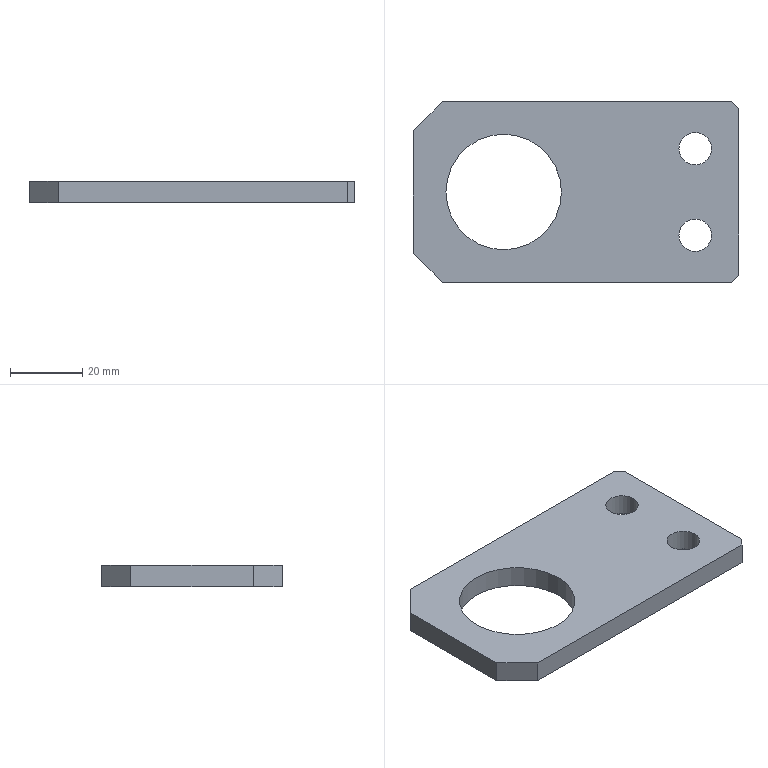Part | NX | features solid 2 | 1 solid | 13 faces | box 90.05 x 50 x 6 mm | volume 21018 mm3 | plane 10 | cylinder 3 | commonest cylinder face diameters 9 x2 32 x1
STEP:
#1=CARTESIAN_POINT('',(1617.788,161.279,-54.));
#2=VERTEX_POINT('',#1);
#3=CARTESIAN_POINT('',(1697.838,161.279,-54.));
#4=VERTEX_POINT('',#3);
#5=CARTESIAN_POINT('',(1655.838,161.279,-54.));
#6=DIRECTION('',(1.,0.,0.));
#7=VECTOR('',#6,1000.);
#8=LINE('',#5,#7);
#9=EDGE_CURVE('',#2,#4,#8,.T.);
#10=ORIENTED_EDGE('',*,*,#9,.F.);
#11=CARTESIAN_POINT('',(1609.788,153.279,-54.));
#12=VERTEX_POINT('',#11);
#13=CARTESIAN_POINT('',(1623.788,167.279,-54.));
#14=DIRECTION('',(0.7071,0.7071,0.));
#15=VECTOR('',#14,1000.);
#16=LINE('',#13,#15);
#17=EDGE_CURVE('',#2,#12,#16,.F.);
#18=ORIENTED_EDGE('',*,*,#17,.T.);
#19=CARTESIAN_POINT('',(1609.788,119.279,-54.));
#20=VERTEX_POINT('',#19);
#21=CARTESIAN_POINT('',(1609.788,136.279,-54.));
#22=DIRECTION('',(0.,1.,0.));
#23=VECTOR('',#22,1000.);
#24=LINE('',#21,#23);
#25=EDGE_CURVE('',#20,#12,#24,.T.);
#26=ORIENTED_EDGE('',*,*,#25,.F.);
#27=CARTESIAN_POINT('',(1617.788,111.279,-54.));
#28=VERTEX_POINT('',#27);
#29=CARTESIAN_POINT('',(1623.788,105.279,-54.));
#30=DIRECTION('',(-0.7071,0.7071,0.));
#31=VECTOR('',#30,1000.);
#32=LINE('',#29,#31);
#33=EDGE_CURVE('',#20,#28,#32,.F.);
#34=ORIENTED_EDGE('',*,*,#33,.T.);
#35=CARTESIAN_POINT('',(1697.838,111.279,-54.));
#36=VERTEX_POINT('',#35);
#37=CARTESIAN_POINT('',(1655.838,111.279,-54.));
#38=DIRECTION('',(-1.,0.,0.));
#39=VECTOR('',#38,1000.);
#40=LINE('',#37,#39);
#41=EDGE_CURVE('',#36,#28,#40,.T.);
#42=ORIENTED_EDGE('',*,*,#41,.F.);
#43=CARTESIAN_POINT('',(1699.838,113.279,-54.));
#44=VERTEX_POINT('',#43);
#45=CARTESIAN_POINT('',(1688.838,102.279,-54.));
#46=DIRECTION('',(-0.7071,-0.7071,0.));
#47=VECTOR('',#46,1000.);
#48=LINE('',#45,#47);
#49=EDGE_CURVE('',#36,#44,#48,.F.);
#50=ORIENTED_EDGE('',*,*,#49,.T.);
#51=CARTESIAN_POINT('',(1699.838,159.279,-54.));
#52=VERTEX_POINT('',#51);
#53=CARTESIAN_POINT('',(1699.838,136.279,-54.));
#54=DIRECTION('',(0.,-1.,0.));
#55=VECTOR('',#54,1000.);
#56=LINE('',#53,#55);
#57=EDGE_CURVE('',#52,#44,#56,.T.);
#58=ORIENTED_EDGE('',*,*,#57,.F.);
#59=CARTESIAN_POINT('',(1688.838,170.279,-54.));
#60=DIRECTION('',(0.7071,-0.7071,0.));
#61=VECTOR('',#60,1000.);
#62=LINE('',#59,#61);
#63=EDGE_CURVE('',#52,#4,#62,.F.);
#64=ORIENTED_EDGE('',*,*,#63,.T.);
#65=EDGE_LOOP('',(#10,#18,#26,#34,#42,#50,#58,#64));
#66=FACE_BOUND('',#65,.T.);
#67=CARTESIAN_POINT('',(1683.338,124.279,-54.));
#68=VERTEX_POINT('',#67);
#69=CARTESIAN_POINT('',(1687.838,124.279,-54.));
#70=DIRECTION('',(0.,0.,-1.));
#71=DIRECTION('',(-1.,0.,0.));
#72=AXIS2_PLACEMENT_3D('',#69,#70,#71);
#73=CIRCLE('',#72,4.5);
#74=EDGE_CURVE('',#68,#68,#73,.T.);
#75=ORIENTED_EDGE('',*,*,#74,.T.);
#76=EDGE_LOOP('',(#75));
#77=FACE_BOUND('',#76,.T.);
#78=CARTESIAN_POINT('',(1683.338,148.279,-54.));
#79=VERTEX_POINT('',#78);
#80=CARTESIAN_POINT('',(1687.838,148.279,-54.));
#81=DIRECTION('',(0.,0.,-1.));
#82=DIRECTION('',(-1.,0.,0.));
#83=AXIS2_PLACEMENT_3D('',#80,#81,#82);
#84=CIRCLE('',#83,4.5);
#85=EDGE_CURVE('',#79,#79,#84,.T.);
#86=ORIENTED_EDGE('',*,*,#85,.T.);
#87=EDGE_LOOP('',(#86));
#88=FACE_BOUND('',#87,.T.);
#89=CARTESIAN_POINT('',(1618.788,136.279,-54.));
#90=VERTEX_POINT('',#89);
#91=CARTESIAN_POINT('',(1634.788,136.279,-54.));
#92=DIRECTION('',(0.,0.,-1.));
#93=DIRECTION('',(-1.,0.,0.));
#94=AXIS2_PLACEMENT_3D('',#91,#92,#93);
#95=CIRCLE('',#94,16.);
#96=EDGE_CURVE('',#90,#90,#95,.T.);
#97=ORIENTED_EDGE('',*,*,#96,.T.);
#98=EDGE_LOOP('',(#97));
#99=FACE_BOUND('',#98,.T.);
#100=CARTESIAN_POINT('',(1655.838,136.279,-54.));
#101=DIRECTION('',(0.,0.,1.));
#102=DIRECTION('',(1.,0.,0.));
#103=AXIS2_PLACEMENT_3D('',#100,#101,#102);
#104=PLANE('',#103);
#105=ADVANCED_FACE('',(#66,#77,#88,#99),#104,.T.);
#106=ORIENTED_EDGE('',*,*,#41,.T.);
#107=CARTESIAN_POINT('',(1617.788,111.279,-60.));
#108=VERTEX_POINT('',#107);
#109=CARTESIAN_POINT('',(1617.788,111.279,-60.));
#110=DIRECTION('',(0.,0.,-1.));
#111=VECTOR('',#110,1000.);
#112=LINE('',#109,#111);
#113=EDGE_CURVE('',#28,#108,#112,.T.);
#114=ORIENTED_EDGE('',*,*,#113,.T.);
#115=CARTESIAN_POINT('',(1697.838,111.279,-60.));
#116=VERTEX_POINT('',#115);
#117=CARTESIAN_POINT('',(1655.838,111.279,-60.));
#118=DIRECTION('',(1.,0.,0.));
#119=VECTOR('',#118,1000.);
#120=LINE('',#117,#119);
#121=EDGE_CURVE('',#108,#116,#120,.T.);
#122=ORIENTED_EDGE('',*,*,#121,.T.);
#123=CARTESIAN_POINT('',(1697.838,111.279,-60.));
#124=DIRECTION('',(0.,0.,1.));
#125=VECTOR('',#124,1000.);
#126=LINE('',#123,#125);
#127=EDGE_CURVE('',#116,#36,#126,.T.);
#128=ORIENTED_EDGE('',*,*,#127,.T.);
#129=EDGE_LOOP('',(#106,#114,#122,#128));
#130=FACE_BOUND('',#129,.T.);
#131=CARTESIAN_POINT('',(1655.838,111.279,-60.));
#132=DIRECTION('',(0.,-1.,0.));
#133=DIRECTION('',(0.,0.,-1.));
#134=AXIS2_PLACEMENT_3D('',#131,#132,#133);
#135=PLANE('',#134);
#136=ADVANCED_FACE('',(#130),#135,.T.);
#137=CARTESIAN_POINT('',(1697.838,161.279,-60.));
#138=VERTEX_POINT('',#137);
#139=CARTESIAN_POINT('',(1617.788,161.279,-60.));
#140=VERTEX_POINT('',#139);
#141=CARTESIAN_POINT('',(1655.838,161.279,-60.));
#142=DIRECTION('',(-1.,0.,0.));
#143=VECTOR('',#142,1000.);
#144=LINE('',#141,#143);
#145=EDGE_CURVE('',#138,#140,#144,.T.);
#146=ORIENTED_EDGE('',*,*,#145,.T.);
#147=CARTESIAN_POINT('',(1617.788,161.279,-60.));
#148=DIRECTION('',(0.,0.,1.));
#149=VECTOR('',#148,1000.);
#150=LINE('',#147,#149);
#151=EDGE_CURVE('',#140,#2,#150,.T.);
#152=ORIENTED_EDGE('',*,*,#151,.T.);
#153=ORIENTED_EDGE('',*,*,#9,.T.);
#154=CARTESIAN_POINT('',(1697.838,161.279,-60.));
#155=DIRECTION('',(0.,0.,-1.));
#156=VECTOR('',#155,1000.);
#157=LINE('',#154,#156);
#158=EDGE_CURVE('',#4,#138,#157,.T.);
#159=ORIENTED_EDGE('',*,*,#158,.T.);
#160=EDGE_LOOP('',(#146,#152,#153,#159));
#161=FACE_BOUND('',#160,.T.);
#162=CARTESIAN_POINT('',(1655.838,161.279,-60.));
#163=DIRECTION('',(0.,1.,0.));
#164=DIRECTION('',(0.,0.,1.));
#165=AXIS2_PLACEMENT_3D('',#162,#163,#164);
#166=PLANE('',#165);
#167=ADVANCED_FACE('',(#161),#166,.T.);
#168=ORIENTED_EDGE('',*,*,#121,.F.);
#169=CARTESIAN_POINT('',(1609.788,119.279,-60.));
#170=VERTEX_POINT('',#169);
#171=CARTESIAN_POINT('',(1623.788,105.279,-60.));
#172=DIRECTION('',(0.7071,-0.7071,0.));
#173=VECTOR('',#172,1000.);
#174=LINE('',#171,#173);
#175=EDGE_CURVE('',#108,#170,#174,.F.);
#176=ORIENTED_EDGE('',*,*,#175,.T.);
#177=CARTESIAN_POINT('',(1609.788,153.279,-60.));
#178=VERTEX_POINT('',#177);
#179=CARTESIAN_POINT('',(1609.788,136.279,-60.));
#180=DIRECTION('',(0.,-1.,0.));
#181=VECTOR('',#180,1000.);
#182=LINE('',#179,#181);
#183=EDGE_CURVE('',#178,#170,#182,.T.);
#184=ORIENTED_EDGE('',*,*,#183,.F.);
#185=CARTESIAN_POINT('',(1623.788,167.279,-60.));
#186=DIRECTION('',(-0.7071,-0.7071,0.));
#187=VECTOR('',#186,1000.);
#188=LINE('',#185,#187);
#189=EDGE_CURVE('',#178,#140,#188,.F.);
#190=ORIENTED_EDGE('',*,*,#189,.T.);
#191=ORIENTED_EDGE('',*,*,#145,.F.);
#192=CARTESIAN_POINT('',(1699.838,159.279,-60.));
#193=VERTEX_POINT('',#192);
#194=CARTESIAN_POINT('',(1688.838,170.279,-60.));
#195=DIRECTION('',(-0.7071,0.7071,0.));
#196=VECTOR('',#195,1000.);
#197=LINE('',#194,#196);
#198=EDGE_CURVE('',#138,#193,#197,.F.);
#199=ORIENTED_EDGE('',*,*,#198,.T.);
#200=CARTESIAN_POINT('',(1699.838,113.279,-60.));
#201=VERTEX_POINT('',#200);
#202=CARTESIAN_POINT('',(1699.838,136.279,-60.));
#203=DIRECTION('',(0.,1.,0.));
#204=VECTOR('',#203,1000.);
#205=LINE('',#202,#204);
#206=EDGE_CURVE('',#201,#193,#205,.T.);
#207=ORIENTED_EDGE('',*,*,#206,.F.);
#208=CARTESIAN_POINT('',(1688.838,102.279,-60.));
#209=DIRECTION('',(0.7071,0.7071,0.));
#210=VECTOR('',#209,1000.);
#211=LINE('',#208,#210);
#212=EDGE_CURVE('',#201,#116,#211,.F.);
#213=ORIENTED_EDGE('',*,*,#212,.T.);
#214=EDGE_LOOP('',(#168,#176,#184,#190,#191,#199,#207,#213));
#215=FACE_BOUND('',#214,.T.);
#216=CARTESIAN_POINT('',(1683.338,124.279,-60.));
#217=VERTEX_POINT('',#216);
#218=CARTESIAN_POINT('',(1687.838,124.279,-60.));
#219=DIRECTION('',(0.,0.,-1.));
#220=DIRECTION('',(-1.,0.,0.));
#221=AXIS2_PLACEMENT_3D('',#218,#219,#220);
#222=CIRCLE('',#221,4.5);
#223=EDGE_CURVE('',#217,#217,#222,.T.);
#224=ORIENTED_EDGE('',*,*,#223,.F.);
#225=EDGE_LOOP('',(#224));
#226=FACE_BOUND('',#225,.T.);
#227=CARTESIAN_POINT('',(1683.338,148.279,-60.));
#228=VERTEX_POINT('',#227);
#229=CARTESIAN_POINT('',(1687.838,148.279,-60.));
#230=DIRECTION('',(0.,0.,-1.));
#231=DIRECTION('',(-1.,0.,0.));
#232=AXIS2_PLACEMENT_3D('',#229,#230,#231);
#233=CIRCLE('',#232,4.5);
#234=EDGE_CURVE('',#228,#228,#233,.T.);
#235=ORIENTED_EDGE('',*,*,#234,.F.);
#236=EDGE_LOOP('',(#235));
#237=FACE_BOUND('',#236,.T.);
#238=CARTESIAN_POINT('',(1618.788,136.279,-60.));
#239=VERTEX_POINT('',#238);
#240=CARTESIAN_POINT('',(1634.788,136.279,-60.));
#241=DIRECTION('',(0.,0.,-1.));
#242=DIRECTION('',(-1.,0.,0.));
#243=AXIS2_PLACEMENT_3D('',#240,#241,#242);
#244=CIRCLE('',#243,16.);
#245=EDGE_CURVE('',#239,#239,#244,.T.);
#246=ORIENTED_EDGE('',*,*,#245,.F.);
#247=EDGE_LOOP('',(#246));
#248=FACE_BOUND('',#247,.T.);
#249=CARTESIAN_POINT('',(1655.838,136.279,-60.));
#250=DIRECTION('',(0.,0.,-1.));
#251=DIRECTION('',(-1.,0.,0.));
#252=AXIS2_PLACEMENT_3D('',#249,#250,#251);
#253=PLANE('',#252);
#254=ADVANCED_FACE('',(#215,#226,#237,#248),#253,.T.);
#255=ORIENTED_EDGE('',*,*,#206,.T.);
#256=CARTESIAN_POINT('',(1699.838,159.279,-60.));
#257=DIRECTION('',(0.,0.,1.));
#258=VECTOR('',#257,1000.);
#259=LINE('',#256,#258);
#260=EDGE_CURVE('',#193,#52,#259,.T.);
#261=ORIENTED_EDGE('',*,*,#260,.T.);
#262=ORIENTED_EDGE('',*,*,#57,.T.);
#263=CARTESIAN_POINT('',(1699.838,113.279,-60.));
#264=DIRECTION('',(0.,0.,-1.));
#265=VECTOR('',#264,1000.);
#266=LINE('',#263,#265);
#267=EDGE_CURVE('',#44,#201,#266,.T.);
#268=ORIENTED_EDGE('',*,*,#267,.T.);
#269=EDGE_LOOP('',(#255,#261,#262,#268));
#270=FACE_BOUND('',#269,.T.);
#271=CARTESIAN_POINT('',(1699.838,136.279,-60.));
#272=DIRECTION('',(1.,0.,0.));
#273=DIRECTION('',(0.,0.,-1.));
#274=AXIS2_PLACEMENT_3D('',#271,#272,#273);
#275=PLANE('',#274);
#276=ADVANCED_FACE('',(#270),#275,.T.);
#277=ORIENTED_EDGE('',*,*,#198,.F.);
#278=ORIENTED_EDGE('',*,*,#158,.F.);
#279=ORIENTED_EDGE('',*,*,#63,.F.);
#280=ORIENTED_EDGE('',*,*,#260,.F.);
#281=EDGE_LOOP('',(#277,#278,#279,#280));
#282=FACE_BOUND('',#281,.T.);
#283=CARTESIAN_POINT('',(1699.838,159.279,-60.));
#284=DIRECTION('',(-0.7071,-0.7071,0.));
#285=DIRECTION('',(0.7071,-0.7071,0.));
#286=AXIS2_PLACEMENT_3D('',#283,#284,#285);
#287=PLANE('',#286);
#288=ADVANCED_FACE('',(#282),#287,.F.);
#289=ORIENTED_EDGE('',*,*,#212,.F.);
#290=ORIENTED_EDGE('',*,*,#267,.F.);
#291=ORIENTED_EDGE('',*,*,#49,.F.);
#292=ORIENTED_EDGE('',*,*,#127,.F.);
#293=EDGE_LOOP('',(#289,#290,#291,#292));
#294=FACE_BOUND('',#293,.T.);
#295=CARTESIAN_POINT('',(1697.838,111.279,-60.));
#296=DIRECTION('',(-0.7071,0.7071,0.));
#297=DIRECTION('',(-0.7071,-0.7071,0.));
#298=AXIS2_PLACEMENT_3D('',#295,#296,#297);
#299=PLANE('',#298);
#300=ADVANCED_FACE('',(#294),#299,.F.);
#301=ORIENTED_EDGE('',*,*,#234,.T.);
#302=EDGE_LOOP('',(#301));
#303=FACE_BOUND('',#302,.T.);
#304=ORIENTED_EDGE('',*,*,#85,.F.);
#305=EDGE_LOOP('',(#304));
#306=FACE_BOUND('',#305,.T.);
#307=CARTESIAN_POINT('',(1687.838,148.279,-54.));
#308=DIRECTION('',(0.,0.,-1.));
#309=DIRECTION('',(-1.,0.,0.));
#310=AXIS2_PLACEMENT_3D('',#307,#308,#309);
#311=CYLINDRICAL_SURFACE('',#310,4.5);
#312=ADVANCED_FACE('',(#303,#306),#311,.F.);
#313=ORIENTED_EDGE('',*,*,#223,.T.);
#314=EDGE_LOOP('',(#313));
#315=FACE_BOUND('',#314,.T.);
#316=ORIENTED_EDGE('',*,*,#74,.F.);
#317=EDGE_LOOP('',(#316));
#318=FACE_BOUND('',#317,.T.);
#319=CARTESIAN_POINT('',(1687.838,124.279,-54.));
#320=DIRECTION('',(0.,0.,-1.));
#321=DIRECTION('',(-1.,0.,0.));
#322=AXIS2_PLACEMENT_3D('',#319,#320,#321);
#323=CYLINDRICAL_SURFACE('',#322,4.5);
#324=ADVANCED_FACE('',(#315,#318),#323,.F.);
#325=ORIENTED_EDGE('',*,*,#189,.F.);
#326=CARTESIAN_POINT('',(1609.788,153.279,-60.));
#327=DIRECTION('',(0.,0.,-1.));
#328=VECTOR('',#327,1000.);
#329=LINE('',#326,#328);
#330=EDGE_CURVE('',#12,#178,#329,.T.);
#331=ORIENTED_EDGE('',*,*,#330,.F.);
#332=ORIENTED_EDGE('',*,*,#17,.F.);
#333=ORIENTED_EDGE('',*,*,#151,.F.);
#334=EDGE_LOOP('',(#325,#331,#332,#333));
#335=FACE_BOUND('',#334,.T.);
#336=CARTESIAN_POINT('',(1617.788,161.279,-60.));
#337=DIRECTION('',(0.7071,-0.7071,0.));
#338=DIRECTION('',(0.7071,0.7071,0.));
#339=AXIS2_PLACEMENT_3D('',#336,#337,#338);
#340=PLANE('',#339);
#341=ADVANCED_FACE('',(#335),#340,.F.);
#342=ORIENTED_EDGE('',*,*,#25,.T.);
#343=ORIENTED_EDGE('',*,*,#330,.T.);
#344=ORIENTED_EDGE('',*,*,#183,.T.);
#345=CARTESIAN_POINT('',(1609.788,119.279,-60.));
#346=DIRECTION('',(0.,0.,1.));
#347=VECTOR('',#346,1000.);
#348=LINE('',#345,#347);
#349=EDGE_CURVE('',#170,#20,#348,.T.);
#350=ORIENTED_EDGE('',*,*,#349,.T.);
#351=EDGE_LOOP('',(#342,#343,#344,#350));
#352=FACE_BOUND('',#351,.T.);
#353=CARTESIAN_POINT('',(1609.788,136.279,-60.));
#354=DIRECTION('',(-1.,0.,0.));
#355=DIRECTION('',(0.,0.,1.));
#356=AXIS2_PLACEMENT_3D('',#353,#354,#355);
#357=PLANE('',#356);
#358=ADVANCED_FACE('',(#352),#357,.T.);
#359=ORIENTED_EDGE('',*,*,#175,.F.);
#360=ORIENTED_EDGE('',*,*,#113,.F.);
#361=ORIENTED_EDGE('',*,*,#33,.F.);
#362=ORIENTED_EDGE('',*,*,#349,.F.);
#363=EDGE_LOOP('',(#359,#360,#361,#362));
#364=FACE_BOUND('',#363,.T.);
#365=CARTESIAN_POINT('',(1609.788,119.279,-60.));
#366=DIRECTION('',(0.7071,0.7071,0.));
#367=DIRECTION('',(-0.7071,0.7071,0.));
#368=AXIS2_PLACEMENT_3D('',#365,#366,#367);
#369=PLANE('',#368);
#370=ADVANCED_FACE('',(#364),#369,.F.);
#371=ORIENTED_EDGE('',*,*,#245,.T.);
#372=EDGE_LOOP('',(#371));
#373=FACE_BOUND('',#372,.T.);
#374=ORIENTED_EDGE('',*,*,#96,.F.);
#375=EDGE_LOOP('',(#374));
#376=FACE_BOUND('',#375,.T.);
#377=CARTESIAN_POINT('',(1634.788,136.279,-54.));
#378=DIRECTION('',(0.,0.,-1.));
#379=DIRECTION('',(-1.,0.,0.));
#380=AXIS2_PLACEMENT_3D('',#377,#378,#379);
#381=CYLINDRICAL_SURFACE('',#380,16.);
#382=ADVANCED_FACE('',(#373,#376),#381,.F.);
#383=CLOSED_SHELL('',(#105,#136,#167,#254,#276,#288,#300,#312,#324,#341,#358,#370,#382));
#384=MANIFOLD_SOLID_BREP('',#383);
#385=(LENGTH_UNIT()NAMED_UNIT(*)SI_UNIT(.MILLI.,.METRE.));
#386=UNCERTAINTY_MEASURE_WITH_UNIT(LENGTH_MEASURE(0.00001),#385,'','');
#387=(NAMED_UNIT(*)PLANE_ANGLE_UNIT()SI_UNIT($,.RADIAN.));
#388=(NAMED_UNIT(*)SI_UNIT($,.STERADIAN.)SOLID_ANGLE_UNIT());
#389=(GEOMETRIC_REPRESENTATION_CONTEXT(3)GLOBAL_UNCERTAINTY_ASSIGNED_CONTEXT((#386))GLOBAL_UNIT_ASSIGNED_CONTEXT((#385,#387,#388))REPRESENTATION_CONTEXT('',''));
#390=ADVANCED_BREP_SHAPE_REPRESENTATION('',(#384),#389);